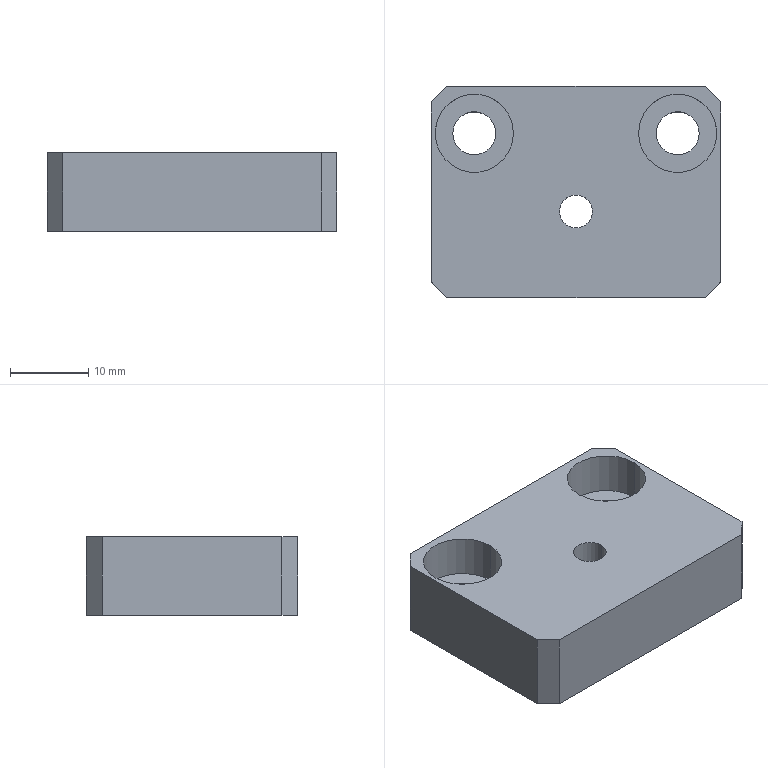Part | SolidWorks | features HoleWzd 2, Chamfer 1, Extrusion 1 | 1 solid | 22 faces | box 37 x 27 x 10 mm | volume 8705 mm3 | plane 12 | cylinder 10 | commonest cylinder face diameters 5.5 x4 10 x4 4.2 x2
STEP:
#1=CARTESIAN_POINT('',(-2.1,-2.5,0.));
#2=VERTEX_POINT('',#1);
#3=CARTESIAN_POINT('',(2.1,-2.5,0.));
#4=VERTEX_POINT('',#3);
#5=CARTESIAN_POINT('',(0.,-2.5,0.));
#6=DIRECTION('',(0.,0.,1.));
#7=DIRECTION('',(1.,0.,0.));
#8=AXIS2_PLACEMENT_3D('',#5,#6,#7);
#9=CIRCLE('',#8,2.1);
#10=EDGE_CURVE('',#2,#4,#9,.T.);
#11=ORIENTED_EDGE('',*,*,#10,.F.);
#12=CARTESIAN_POINT('',(-2.1,-2.5,10.));
#13=VERTEX_POINT('',#12);
#14=CARTESIAN_POINT('',(-2.1,-2.5,10.));
#15=DIRECTION('',(0.,0.,1.));
#16=VECTOR('',#15,1000.);
#17=LINE('',#14,#16);
#18=EDGE_CURVE('',#2,#13,#17,.T.);
#19=ORIENTED_EDGE('',*,*,#18,.T.);
#20=CARTESIAN_POINT('',(2.1,-2.5,10.));
#21=VERTEX_POINT('',#20);
#22=CARTESIAN_POINT('',(0.,-2.5,10.));
#23=DIRECTION('',(0.,0.,1.));
#24=DIRECTION('',(1.,0.,0.));
#25=AXIS2_PLACEMENT_3D('',#22,#23,#24);
#26=CIRCLE('',#25,2.1);
#27=EDGE_CURVE('',#13,#21,#26,.T.);
#28=ORIENTED_EDGE('',*,*,#27,.T.);
#29=CARTESIAN_POINT('',(2.1,-2.5,10.));
#30=DIRECTION('',(0.,0.,1.));
#31=VECTOR('',#30,1000.);
#32=LINE('',#29,#31);
#33=EDGE_CURVE('',#4,#21,#32,.T.);
#34=ORIENTED_EDGE('',*,*,#33,.F.);
#35=EDGE_LOOP('',(#11,#19,#28,#34));
#36=FACE_OUTER_BOUND('',#35,.T.);
#37=CARTESIAN_POINT('',(0.,-2.5,10.));
#38=DIRECTION('',(0.,0.,1.));
#39=DIRECTION('',(1.,0.,0.));
#40=AXIS2_PLACEMENT_3D('',#37,#38,#39);
#41=CYLINDRICAL_SURFACE('',#40,2.1);
#42=ADVANCED_FACE('',(#36),#41,.F.);
#43=CARTESIAN_POINT('',(-18.,7.5,4.6));
#44=VERTEX_POINT('',#43);
#45=CARTESIAN_POINT('',(-8.,7.5,4.6));
#46=VERTEX_POINT('',#45);
#47=CARTESIAN_POINT('',(-13.,7.5,4.6));
#48=DIRECTION('',(0.,0.,1.));
#49=DIRECTION('',(1.,0.,0.));
#50=AXIS2_PLACEMENT_3D('',#47,#48,#49);
#51=CIRCLE('',#50,5.);
#52=EDGE_CURVE('',#44,#46,#51,.T.);
#53=ORIENTED_EDGE('',*,*,#52,.F.);
#54=CARTESIAN_POINT('',(-18.,7.5,10.));
#55=VERTEX_POINT('',#54);
#56=CARTESIAN_POINT('',(-18.,7.5,10.));
#57=DIRECTION('',(0.,0.,1.));
#58=VECTOR('',#57,1000.);
#59=LINE('',#56,#58);
#60=EDGE_CURVE('',#44,#55,#59,.T.);
#61=ORIENTED_EDGE('',*,*,#60,.T.);
#62=CARTESIAN_POINT('',(-8.,7.5,10.));
#63=VERTEX_POINT('',#62);
#64=CARTESIAN_POINT('',(-13.,7.5,10.));
#65=DIRECTION('',(0.,0.,1.));
#66=DIRECTION('',(1.,0.,0.));
#67=AXIS2_PLACEMENT_3D('',#64,#65,#66);
#68=CIRCLE('',#67,5.);
#69=EDGE_CURVE('',#55,#63,#68,.T.);
#70=ORIENTED_EDGE('',*,*,#69,.T.);
#71=CARTESIAN_POINT('',(-8.,7.5,10.));
#72=DIRECTION('',(0.,0.,1.));
#73=VECTOR('',#72,1000.);
#74=LINE('',#71,#73);
#75=EDGE_CURVE('',#46,#63,#74,.T.);
#76=ORIENTED_EDGE('',*,*,#75,.F.);
#77=EDGE_LOOP('',(#53,#61,#70,#76));
#78=FACE_OUTER_BOUND('',#77,.T.);
#79=CARTESIAN_POINT('',(-13.,7.5,10.));
#80=DIRECTION('',(0.,0.,1.));
#81=DIRECTION('',(1.,0.,0.));
#82=AXIS2_PLACEMENT_3D('',#79,#80,#81);
#83=CYLINDRICAL_SURFACE('',#82,5.);
#84=ADVANCED_FACE('',(#78),#83,.F.);
#85=CARTESIAN_POINT('',(-15.75,7.5,0.));
#86=VERTEX_POINT('',#85);
#87=CARTESIAN_POINT('',(-10.25,7.5,0.));
#88=VERTEX_POINT('',#87);
#89=CARTESIAN_POINT('',(-13.,7.5,0.));
#90=DIRECTION('',(0.,0.,1.));
#91=DIRECTION('',(1.,0.,0.));
#92=AXIS2_PLACEMENT_3D('',#89,#90,#91);
#93=CIRCLE('',#92,2.75);
#94=EDGE_CURVE('',#86,#88,#93,.T.);
#95=ORIENTED_EDGE('',*,*,#94,.F.);
#96=CARTESIAN_POINT('',(-15.75,7.5,4.6));
#97=VERTEX_POINT('',#96);
#98=CARTESIAN_POINT('',(-15.75,7.5,10.));
#99=DIRECTION('',(0.,0.,1.));
#100=VECTOR('',#99,1000.);
#101=LINE('',#98,#100);
#102=EDGE_CURVE('',#86,#97,#101,.T.);
#103=ORIENTED_EDGE('',*,*,#102,.T.);
#104=CARTESIAN_POINT('',(-10.25,7.5,4.6));
#105=VERTEX_POINT('',#104);
#106=CARTESIAN_POINT('',(-13.,7.5,4.6));
#107=DIRECTION('',(0.,0.,1.));
#108=DIRECTION('',(1.,0.,0.));
#109=AXIS2_PLACEMENT_3D('',#106,#107,#108);
#110=CIRCLE('',#109,2.75);
#111=EDGE_CURVE('',#97,#105,#110,.T.);
#112=ORIENTED_EDGE('',*,*,#111,.T.);
#113=CARTESIAN_POINT('',(-10.25,7.5,10.));
#114=DIRECTION('',(0.,0.,1.));
#115=VECTOR('',#114,1000.);
#116=LINE('',#113,#115);
#117=EDGE_CURVE('',#88,#105,#116,.T.);
#118=ORIENTED_EDGE('',*,*,#117,.F.);
#119=EDGE_LOOP('',(#95,#103,#112,#118));
#120=FACE_OUTER_BOUND('',#119,.T.);
#121=CARTESIAN_POINT('',(-13.,7.5,10.));
#122=DIRECTION('',(0.,0.,1.));
#123=DIRECTION('',(1.,0.,0.));
#124=AXIS2_PLACEMENT_3D('',#121,#122,#123);
#125=CYLINDRICAL_SURFACE('',#124,2.75);
#126=ADVANCED_FACE('',(#120),#125,.F.);
#127=CARTESIAN_POINT('',(8.,7.5,4.6));
#128=VERTEX_POINT('',#127);
#129=CARTESIAN_POINT('',(18.,7.5,4.6));
#130=VERTEX_POINT('',#129);
#131=CARTESIAN_POINT('',(13.,7.5,4.6));
#132=DIRECTION('',(0.,0.,1.));
#133=DIRECTION('',(1.,0.,0.));
#134=AXIS2_PLACEMENT_3D('',#131,#132,#133);
#135=CIRCLE('',#134,5.);
#136=EDGE_CURVE('',#128,#130,#135,.T.);
#137=ORIENTED_EDGE('',*,*,#136,.F.);
#138=CARTESIAN_POINT('',(8.,7.5,10.));
#139=VERTEX_POINT('',#138);
#140=CARTESIAN_POINT('',(8.,7.5,10.));
#141=DIRECTION('',(0.,0.,1.));
#142=VECTOR('',#141,1000.);
#143=LINE('',#140,#142);
#144=EDGE_CURVE('',#128,#139,#143,.T.);
#145=ORIENTED_EDGE('',*,*,#144,.T.);
#146=CARTESIAN_POINT('',(18.,7.5,10.));
#147=VERTEX_POINT('',#146);
#148=CARTESIAN_POINT('',(13.,7.5,10.));
#149=DIRECTION('',(0.,0.,1.));
#150=DIRECTION('',(1.,0.,0.));
#151=AXIS2_PLACEMENT_3D('',#148,#149,#150);
#152=CIRCLE('',#151,5.);
#153=EDGE_CURVE('',#139,#147,#152,.T.);
#154=ORIENTED_EDGE('',*,*,#153,.T.);
#155=CARTESIAN_POINT('',(18.,7.5,10.));
#156=DIRECTION('',(0.,0.,1.));
#157=VECTOR('',#156,1000.);
#158=LINE('',#155,#157);
#159=EDGE_CURVE('',#130,#147,#158,.T.);
#160=ORIENTED_EDGE('',*,*,#159,.F.);
#161=EDGE_LOOP('',(#137,#145,#154,#160));
#162=FACE_OUTER_BOUND('',#161,.T.);
#163=CARTESIAN_POINT('',(13.,7.5,10.));
#164=DIRECTION('',(0.,0.,1.));
#165=DIRECTION('',(1.,0.,0.));
#166=AXIS2_PLACEMENT_3D('',#163,#164,#165);
#167=CYLINDRICAL_SURFACE('',#166,5.);
#168=ADVANCED_FACE('',(#162),#167,.F.);
#169=CARTESIAN_POINT('',(10.25,7.5,0.));
#170=VERTEX_POINT('',#169);
#171=CARTESIAN_POINT('',(15.75,7.5,0.));
#172=VERTEX_POINT('',#171);
#173=CARTESIAN_POINT('',(13.,7.5,0.));
#174=DIRECTION('',(0.,0.,1.));
#175=DIRECTION('',(1.,0.,0.));
#176=AXIS2_PLACEMENT_3D('',#173,#174,#175);
#177=CIRCLE('',#176,2.75);
#178=EDGE_CURVE('',#170,#172,#177,.T.);
#179=ORIENTED_EDGE('',*,*,#178,.F.);
#180=CARTESIAN_POINT('',(10.25,7.5,4.6));
#181=VERTEX_POINT('',#180);
#182=CARTESIAN_POINT('',(10.25,7.5,10.));
#183=DIRECTION('',(0.,0.,1.));
#184=VECTOR('',#183,1000.);
#185=LINE('',#182,#184);
#186=EDGE_CURVE('',#170,#181,#185,.T.);
#187=ORIENTED_EDGE('',*,*,#186,.T.);
#188=CARTESIAN_POINT('',(15.75,7.5,4.6));
#189=VERTEX_POINT('',#188);
#190=CARTESIAN_POINT('',(13.,7.5,4.6));
#191=DIRECTION('',(0.,0.,1.));
#192=DIRECTION('',(1.,0.,0.));
#193=AXIS2_PLACEMENT_3D('',#190,#191,#192);
#194=CIRCLE('',#193,2.75);
#195=EDGE_CURVE('',#181,#189,#194,.T.);
#196=ORIENTED_EDGE('',*,*,#195,.T.);
#197=CARTESIAN_POINT('',(15.75,7.5,10.));
#198=DIRECTION('',(0.,0.,1.));
#199=VECTOR('',#198,1000.);
#200=LINE('',#197,#199);
#201=EDGE_CURVE('',#172,#189,#200,.T.);
#202=ORIENTED_EDGE('',*,*,#201,.F.);
#203=EDGE_LOOP('',(#179,#187,#196,#202));
#204=FACE_OUTER_BOUND('',#203,.T.);
#205=CARTESIAN_POINT('',(13.,7.5,10.));
#206=DIRECTION('',(0.,0.,1.));
#207=DIRECTION('',(1.,0.,0.));
#208=AXIS2_PLACEMENT_3D('',#205,#206,#207);
#209=CYLINDRICAL_SURFACE('',#208,2.75);
#210=ADVANCED_FACE('',(#204),#209,.F.);
#211=CARTESIAN_POINT('',(18.5,-11.5,10.));
#212=VERTEX_POINT('',#211);
#213=CARTESIAN_POINT('',(18.5,11.5,10.));
#214=VERTEX_POINT('',#213);
#215=CARTESIAN_POINT('',(18.5,13.5,10.));
#216=DIRECTION('',(0.,1.,0.));
#217=VECTOR('',#216,1000.);
#218=LINE('',#215,#217);
#219=EDGE_CURVE('',#212,#214,#218,.T.);
#220=ORIENTED_EDGE('',*,*,#219,.F.);
#221=CARTESIAN_POINT('',(18.5,-11.5,0.));
#222=VERTEX_POINT('',#221);
#223=CARTESIAN_POINT('',(18.5,-11.5,10.));
#224=DIRECTION('',(0.,0.,-1.));
#225=VECTOR('',#224,1000.);
#226=LINE('',#223,#225);
#227=EDGE_CURVE('',#212,#222,#226,.T.);
#228=ORIENTED_EDGE('',*,*,#227,.T.);
#229=CARTESIAN_POINT('',(18.5,11.5,0.));
#230=VERTEX_POINT('',#229);
#231=CARTESIAN_POINT('',(18.5,13.5,0.));
#232=DIRECTION('',(0.,1.,0.));
#233=VECTOR('',#232,1000.);
#234=LINE('',#231,#233);
#235=EDGE_CURVE('',#222,#230,#234,.T.);
#236=ORIENTED_EDGE('',*,*,#235,.T.);
#237=CARTESIAN_POINT('',(18.5,11.5,10.));
#238=DIRECTION('',(0.,0.,1.));
#239=VECTOR('',#238,1000.);
#240=LINE('',#237,#239);
#241=EDGE_CURVE('',#230,#214,#240,.T.);
#242=ORIENTED_EDGE('',*,*,#241,.T.);
#243=EDGE_LOOP('',(#220,#228,#236,#242));
#244=FACE_OUTER_BOUND('',#243,.T.);
#245=CARTESIAN_POINT('',(18.5,13.5,10.));
#246=DIRECTION('',(-1.,0.,0.));
#247=DIRECTION('',(0.,-1.,0.));
#248=AXIS2_PLACEMENT_3D('',#245,#246,#247);
#249=PLANE('',#248);
#250=ADVANCED_FACE('',(#244),#249,.F.);
#251=CARTESIAN_POINT('',(16.5,13.5,10.));
#252=VERTEX_POINT('',#251);
#253=CARTESIAN_POINT('',(-16.5,13.5,10.));
#254=VERTEX_POINT('',#253);
#255=CARTESIAN_POINT('',(-18.5,13.5,10.));
#256=DIRECTION('',(-1.,0.,0.));
#257=VECTOR('',#256,1000.);
#258=LINE('',#255,#257);
#259=EDGE_CURVE('',#252,#254,#258,.T.);
#260=ORIENTED_EDGE('',*,*,#259,.F.);
#261=CARTESIAN_POINT('',(16.5,13.5,0.));
#262=VERTEX_POINT('',#261);
#263=CARTESIAN_POINT('',(16.5,13.5,10.));
#264=DIRECTION('',(0.,0.,-1.));
#265=VECTOR('',#264,1000.);
#266=LINE('',#263,#265);
#267=EDGE_CURVE('',#252,#262,#266,.T.);
#268=ORIENTED_EDGE('',*,*,#267,.T.);
#269=CARTESIAN_POINT('',(-16.5,13.5,0.));
#270=VERTEX_POINT('',#269);
#271=CARTESIAN_POINT('',(-18.5,13.5,0.));
#272=DIRECTION('',(-1.,0.,0.));
#273=VECTOR('',#272,1000.);
#274=LINE('',#271,#273);
#275=EDGE_CURVE('',#262,#270,#274,.T.);
#276=ORIENTED_EDGE('',*,*,#275,.T.);
#277=CARTESIAN_POINT('',(-16.5,13.5,10.));
#278=DIRECTION('',(0.,0.,1.));
#279=VECTOR('',#278,1000.);
#280=LINE('',#277,#279);
#281=EDGE_CURVE('',#270,#254,#280,.T.);
#282=ORIENTED_EDGE('',*,*,#281,.T.);
#283=EDGE_LOOP('',(#260,#268,#276,#282));
#284=FACE_OUTER_BOUND('',#283,.T.);
#285=CARTESIAN_POINT('',(-18.5,13.5,10.));
#286=DIRECTION('',(0.,-1.,0.));
#287=DIRECTION('',(0.,0.,-1.));
#288=AXIS2_PLACEMENT_3D('',#285,#286,#287);
#289=PLANE('',#288);
#290=ADVANCED_FACE('',(#284),#289,.F.);
#291=CARTESIAN_POINT('',(-18.5,11.5,0.));
#292=VERTEX_POINT('',#291);
#293=CARTESIAN_POINT('',(-18.5,-11.5,0.));
#294=VERTEX_POINT('',#293);
#295=CARTESIAN_POINT('',(-18.5,13.5,0.));
#296=DIRECTION('',(0.,-1.,0.));
#297=VECTOR('',#296,1000.);
#298=LINE('',#295,#297);
#299=EDGE_CURVE('',#292,#294,#298,.T.);
#300=ORIENTED_EDGE('',*,*,#299,.T.);
#301=CARTESIAN_POINT('',(-18.5,-11.5,10.));
#302=VERTEX_POINT('',#301);
#303=CARTESIAN_POINT('',(-18.5,-11.5,10.));
#304=DIRECTION('',(0.,0.,1.));
#305=VECTOR('',#304,1000.);
#306=LINE('',#303,#305);
#307=EDGE_CURVE('',#294,#302,#306,.T.);
#308=ORIENTED_EDGE('',*,*,#307,.T.);
#309=CARTESIAN_POINT('',(-18.5,11.5,10.));
#310=VERTEX_POINT('',#309);
#311=CARTESIAN_POINT('',(-18.5,13.5,10.));
#312=DIRECTION('',(0.,-1.,0.));
#313=VECTOR('',#312,1000.);
#314=LINE('',#311,#313);
#315=EDGE_CURVE('',#310,#302,#314,.T.);
#316=ORIENTED_EDGE('',*,*,#315,.F.);
#317=CARTESIAN_POINT('',(-18.5,11.5,10.));
#318=DIRECTION('',(0.,0.,-1.));
#319=VECTOR('',#318,1000.);
#320=LINE('',#317,#319);
#321=EDGE_CURVE('',#310,#292,#320,.T.);
#322=ORIENTED_EDGE('',*,*,#321,.T.);
#323=EDGE_LOOP('',(#300,#308,#316,#322));
#324=FACE_OUTER_BOUND('',#323,.T.);
#325=CARTESIAN_POINT('',(-18.5,13.5,10.));
#326=DIRECTION('',(1.,0.,0.));
#327=DIRECTION('',(0.,1.,0.));
#328=AXIS2_PLACEMENT_3D('',#325,#326,#327);
#329=PLANE('',#328);
#330=ADVANCED_FACE('',(#324),#329,.F.);
#331=CARTESIAN_POINT('',(-16.5,-13.5,10.));
#332=VERTEX_POINT('',#331);
#333=CARTESIAN_POINT('',(16.5,-13.5,10.));
#334=VERTEX_POINT('',#333);
#335=CARTESIAN_POINT('',(-18.5,-13.5,10.));
#336=DIRECTION('',(1.,0.,0.));
#337=VECTOR('',#336,1000.);
#338=LINE('',#335,#337);
#339=EDGE_CURVE('',#332,#334,#338,.T.);
#340=ORIENTED_EDGE('',*,*,#339,.F.);
#341=CARTESIAN_POINT('',(-16.5,-13.5,0.));
#342=VERTEX_POINT('',#341);
#343=CARTESIAN_POINT('',(-16.5,-13.5,10.));
#344=DIRECTION('',(0.,0.,-1.));
#345=VECTOR('',#344,1000.);
#346=LINE('',#343,#345);
#347=EDGE_CURVE('',#332,#342,#346,.T.);
#348=ORIENTED_EDGE('',*,*,#347,.T.);
#349=CARTESIAN_POINT('',(16.5,-13.5,0.));
#350=VERTEX_POINT('',#349);
#351=CARTESIAN_POINT('',(-18.5,-13.5,0.));
#352=DIRECTION('',(1.,0.,0.));
#353=VECTOR('',#352,1000.);
#354=LINE('',#351,#353);
#355=EDGE_CURVE('',#342,#350,#354,.T.);
#356=ORIENTED_EDGE('',*,*,#355,.T.);
#357=CARTESIAN_POINT('',(16.5,-13.5,10.));
#358=DIRECTION('',(0.,0.,1.));
#359=VECTOR('',#358,1000.);
#360=LINE('',#357,#359);
#361=EDGE_CURVE('',#350,#334,#360,.T.);
#362=ORIENTED_EDGE('',*,*,#361,.T.);
#363=EDGE_LOOP('',(#340,#348,#356,#362));
#364=FACE_OUTER_BOUND('',#363,.T.);
#365=CARTESIAN_POINT('',(-18.5,-13.5,10.));
#366=DIRECTION('',(0.,1.,0.));
#367=DIRECTION('',(0.,0.,1.));
#368=AXIS2_PLACEMENT_3D('',#365,#366,#367);
#369=PLANE('',#368);
#370=ADVANCED_FACE('',(#364),#369,.F.);
#371=CARTESIAN_POINT('',(0.,-2.5,10.));
#372=DIRECTION('',(0.,0.,1.));
#373=DIRECTION('',(1.,0.,0.));
#374=AXIS2_PLACEMENT_3D('',#371,#372,#373);
#375=CIRCLE('',#374,2.1);
#376=EDGE_CURVE('',#21,#13,#375,.T.);
#377=ORIENTED_EDGE('',*,*,#376,.F.);
#378=ORIENTED_EDGE('',*,*,#27,.F.);
#379=EDGE_LOOP('',(#377,#378));
#380=FACE_BOUND('',#379,.T.);
#381=CARTESIAN_POINT('',(-13.,7.5,10.));
#382=DIRECTION('',(0.,0.,1.));
#383=DIRECTION('',(1.,0.,0.));
#384=AXIS2_PLACEMENT_3D('',#381,#382,#383);
#385=CIRCLE('',#384,5.);
#386=EDGE_CURVE('',#63,#55,#385,.T.);
#387=ORIENTED_EDGE('',*,*,#386,.F.);
#388=ORIENTED_EDGE('',*,*,#69,.F.);
#389=EDGE_LOOP('',(#387,#388));
#390=FACE_BOUND('',#389,.T.);
#391=CARTESIAN_POINT('',(13.,7.5,10.));
#392=DIRECTION('',(0.,0.,1.));
#393=DIRECTION('',(1.,0.,0.));
#394=AXIS2_PLACEMENT_3D('',#391,#392,#393);
#395=CIRCLE('',#394,5.);
#396=EDGE_CURVE('',#147,#139,#395,.T.);
#397=ORIENTED_EDGE('',*,*,#396,.F.);
#398=ORIENTED_EDGE('',*,*,#153,.F.);
#399=EDGE_LOOP('',(#397,#398));
#400=FACE_BOUND('',#399,.T.);
#401=ORIENTED_EDGE('',*,*,#315,.T.);
#402=CARTESIAN_POINT('',(-15.,-15.,10.));
#403=DIRECTION('',(0.7071,-0.7071,0.));
#404=VECTOR('',#403,1000.);
#405=LINE('',#402,#404);
#406=EDGE_CURVE('',#302,#332,#405,.T.);
#407=ORIENTED_EDGE('',*,*,#406,.T.);
#408=ORIENTED_EDGE('',*,*,#339,.T.);
#409=CARTESIAN_POINT('',(15.,-15.,10.));
#410=DIRECTION('',(0.7071,0.7071,0.));
#411=VECTOR('',#410,1000.);
#412=LINE('',#409,#411);
#413=EDGE_CURVE('',#334,#212,#412,.T.);
#414=ORIENTED_EDGE('',*,*,#413,.T.);
#415=ORIENTED_EDGE('',*,*,#219,.T.);
#416=CARTESIAN_POINT('',(15.,15.,10.));
#417=DIRECTION('',(-0.7071,0.7071,0.));
#418=VECTOR('',#417,1000.);
#419=LINE('',#416,#418);
#420=EDGE_CURVE('',#214,#252,#419,.T.);
#421=ORIENTED_EDGE('',*,*,#420,.T.);
#422=ORIENTED_EDGE('',*,*,#259,.T.);
#423=CARTESIAN_POINT('',(-15.,15.,10.));
#424=DIRECTION('',(-0.7071,-0.7071,0.));
#425=VECTOR('',#424,1000.);
#426=LINE('',#423,#425);
#427=EDGE_CURVE('',#254,#310,#426,.T.);
#428=ORIENTED_EDGE('',*,*,#427,.T.);
#429=EDGE_LOOP('',(#401,#407,#408,#414,#415,#421,#422,#428));
#430=FACE_OUTER_BOUND('',#429,.T.);
#431=CARTESIAN_POINT('',(0.,0.,10.));
#432=DIRECTION('',(0.,0.,1.));
#433=DIRECTION('',(1.,0.,0.));
#434=AXIS2_PLACEMENT_3D('',#431,#432,#433);
#435=PLANE('',#434);
#436=ADVANCED_FACE('',(#380,#390,#400,#430),#435,.T.);
#437=CARTESIAN_POINT('',(0.,-2.5,0.));
#438=DIRECTION('',(0.,0.,1.));
#439=DIRECTION('',(1.,0.,0.));
#440=AXIS2_PLACEMENT_3D('',#437,#438,#439);
#441=CIRCLE('',#440,2.1);
#442=EDGE_CURVE('',#4,#2,#441,.T.);
#443=ORIENTED_EDGE('',*,*,#442,.T.);
#444=ORIENTED_EDGE('',*,*,#10,.T.);
#445=EDGE_LOOP('',(#443,#444));
#446=FACE_BOUND('',#445,.T.);
#447=CARTESIAN_POINT('',(-13.,7.5,0.));
#448=DIRECTION('',(0.,0.,1.));
#449=DIRECTION('',(1.,0.,0.));
#450=AXIS2_PLACEMENT_3D('',#447,#448,#449);
#451=CIRCLE('',#450,2.75);
#452=EDGE_CURVE('',#88,#86,#451,.T.);
#453=ORIENTED_EDGE('',*,*,#452,.T.);
#454=ORIENTED_EDGE('',*,*,#94,.T.);
#455=EDGE_LOOP('',(#453,#454));
#456=FACE_BOUND('',#455,.T.);
#457=CARTESIAN_POINT('',(13.,7.5,0.));
#458=DIRECTION('',(0.,0.,1.));
#459=DIRECTION('',(1.,0.,0.));
#460=AXIS2_PLACEMENT_3D('',#457,#458,#459);
#461=CIRCLE('',#460,2.75);
#462=EDGE_CURVE('',#172,#170,#461,.T.);
#463=ORIENTED_EDGE('',*,*,#462,.T.);
#464=ORIENTED_EDGE('',*,*,#178,.T.);
#465=EDGE_LOOP('',(#463,#464));
#466=FACE_BOUND('',#465,.T.);
#467=ORIENTED_EDGE('',*,*,#355,.F.);
#468=CARTESIAN_POINT('',(-16.5,-13.5,0.));
#469=DIRECTION('',(-0.7071,0.7071,0.));
#470=VECTOR('',#469,1000.);
#471=LINE('',#468,#470);
#472=EDGE_CURVE('',#342,#294,#471,.T.);
#473=ORIENTED_EDGE('',*,*,#472,.T.);
#474=ORIENTED_EDGE('',*,*,#299,.F.);
#475=CARTESIAN_POINT('',(-18.5,11.5,0.));
#476=DIRECTION('',(0.7071,0.7071,0.));
#477=VECTOR('',#476,1000.);
#478=LINE('',#475,#477);
#479=EDGE_CURVE('',#292,#270,#478,.T.);
#480=ORIENTED_EDGE('',*,*,#479,.T.);
#481=ORIENTED_EDGE('',*,*,#275,.F.);
#482=CARTESIAN_POINT('',(16.5,13.5,0.));
#483=DIRECTION('',(0.7071,-0.7071,0.));
#484=VECTOR('',#483,1000.);
#485=LINE('',#482,#484);
#486=EDGE_CURVE('',#262,#230,#485,.T.);
#487=ORIENTED_EDGE('',*,*,#486,.T.);
#488=ORIENTED_EDGE('',*,*,#235,.F.);
#489=CARTESIAN_POINT('',(18.5,-11.5,0.));
#490=DIRECTION('',(-0.7071,-0.7071,0.));
#491=VECTOR('',#490,1000.);
#492=LINE('',#489,#491);
#493=EDGE_CURVE('',#222,#350,#492,.T.);
#494=ORIENTED_EDGE('',*,*,#493,.T.);
#495=EDGE_LOOP('',(#467,#473,#474,#480,#481,#487,#488,#494));
#496=FACE_OUTER_BOUND('',#495,.T.);
#497=CARTESIAN_POINT('',(0.,0.,0.));
#498=DIRECTION('',(0.,0.,1.));
#499=DIRECTION('',(1.,0.,0.));
#500=AXIS2_PLACEMENT_3D('',#497,#498,#499);
#501=PLANE('',#500);
#502=ADVANCED_FACE('',(#446,#456,#466,#496),#501,.F.);
#503=ORIENTED_EDGE('',*,*,#186,.F.);
#504=ORIENTED_EDGE('',*,*,#462,.F.);
#505=ORIENTED_EDGE('',*,*,#201,.T.);
#506=CARTESIAN_POINT('',(13.,7.5,4.6));
#507=DIRECTION('',(0.,0.,1.));
#508=DIRECTION('',(1.,0.,0.));
#509=AXIS2_PLACEMENT_3D('',#506,#507,#508);
#510=CIRCLE('',#509,2.75);
#511=EDGE_CURVE('',#189,#181,#510,.T.);
#512=ORIENTED_EDGE('',*,*,#511,.T.);
#513=EDGE_LOOP('',(#503,#504,#505,#512));
#514=FACE_OUTER_BOUND('',#513,.T.);
#515=CARTESIAN_POINT('',(13.,7.5,10.));
#516=DIRECTION('',(0.,0.,1.));
#517=DIRECTION('',(1.,0.,0.));
#518=AXIS2_PLACEMENT_3D('',#515,#516,#517);
#519=CYLINDRICAL_SURFACE('',#518,2.75);
#520=ADVANCED_FACE('',(#514),#519,.F.);
#521=ORIENTED_EDGE('',*,*,#511,.F.);
#522=ORIENTED_EDGE('',*,*,#195,.F.);
#523=EDGE_LOOP('',(#521,#522));
#524=FACE_BOUND('',#523,.T.);
#525=CARTESIAN_POINT('',(13.,7.5,4.6));
#526=DIRECTION('',(0.,0.,1.));
#527=DIRECTION('',(1.,0.,0.));
#528=AXIS2_PLACEMENT_3D('',#525,#526,#527);
#529=CIRCLE('',#528,5.);
#530=EDGE_CURVE('',#130,#128,#529,.T.);
#531=ORIENTED_EDGE('',*,*,#530,.T.);
#532=ORIENTED_EDGE('',*,*,#136,.T.);
#533=EDGE_LOOP('',(#531,#532));
#534=FACE_OUTER_BOUND('',#533,.T.);
#535=CARTESIAN_POINT('',(15.75,7.5,4.6));
#536=DIRECTION('',(0.,0.,-1.));
#537=DIRECTION('',(-1.,0.,0.));
#538=AXIS2_PLACEMENT_3D('',#535,#536,#537);
#539=PLANE('',#538);
#540=ADVANCED_FACE('',(#524,#534),#539,.F.);
#541=ORIENTED_EDGE('',*,*,#144,.F.);
#542=ORIENTED_EDGE('',*,*,#530,.F.);
#543=ORIENTED_EDGE('',*,*,#159,.T.);
#544=ORIENTED_EDGE('',*,*,#396,.T.);
#545=EDGE_LOOP('',(#541,#542,#543,#544));
#546=FACE_OUTER_BOUND('',#545,.T.);
#547=CARTESIAN_POINT('',(13.,7.5,10.));
#548=DIRECTION('',(0.,0.,1.));
#549=DIRECTION('',(1.,0.,0.));
#550=AXIS2_PLACEMENT_3D('',#547,#548,#549);
#551=CYLINDRICAL_SURFACE('',#550,5.);
#552=ADVANCED_FACE('',(#546),#551,.F.);
#553=ORIENTED_EDGE('',*,*,#102,.F.);
#554=ORIENTED_EDGE('',*,*,#452,.F.);
#555=ORIENTED_EDGE('',*,*,#117,.T.);
#556=CARTESIAN_POINT('',(-13.,7.5,4.6));
#557=DIRECTION('',(0.,0.,1.));
#558=DIRECTION('',(1.,0.,0.));
#559=AXIS2_PLACEMENT_3D('',#556,#557,#558);
#560=CIRCLE('',#559,2.75);
#561=EDGE_CURVE('',#105,#97,#560,.T.);
#562=ORIENTED_EDGE('',*,*,#561,.T.);
#563=EDGE_LOOP('',(#553,#554,#555,#562));
#564=FACE_OUTER_BOUND('',#563,.T.);
#565=CARTESIAN_POINT('',(-13.,7.5,10.));
#566=DIRECTION('',(0.,0.,1.));
#567=DIRECTION('',(1.,0.,0.));
#568=AXIS2_PLACEMENT_3D('',#565,#566,#567);
#569=CYLINDRICAL_SURFACE('',#568,2.75);
#570=ADVANCED_FACE('',(#564),#569,.F.);
#571=ORIENTED_EDGE('',*,*,#561,.F.);
#572=ORIENTED_EDGE('',*,*,#111,.F.);
#573=EDGE_LOOP('',(#571,#572));
#574=FACE_BOUND('',#573,.T.);
#575=CARTESIAN_POINT('',(-13.,7.5,4.6));
#576=DIRECTION('',(0.,0.,1.));
#577=DIRECTION('',(1.,0.,0.));
#578=AXIS2_PLACEMENT_3D('',#575,#576,#577);
#579=CIRCLE('',#578,5.);
#580=EDGE_CURVE('',#46,#44,#579,.T.);
#581=ORIENTED_EDGE('',*,*,#580,.T.);
#582=ORIENTED_EDGE('',*,*,#52,.T.);
#583=EDGE_LOOP('',(#581,#582));
#584=FACE_OUTER_BOUND('',#583,.T.);
#585=CARTESIAN_POINT('',(-10.25,7.5,4.6));
#586=DIRECTION('',(0.,0.,-1.));
#587=DIRECTION('',(-1.,0.,0.));
#588=AXIS2_PLACEMENT_3D('',#585,#586,#587);
#589=PLANE('',#588);
#590=ADVANCED_FACE('',(#574,#584),#589,.F.);
#591=ORIENTED_EDGE('',*,*,#60,.F.);
#592=ORIENTED_EDGE('',*,*,#580,.F.);
#593=ORIENTED_EDGE('',*,*,#75,.T.);
#594=ORIENTED_EDGE('',*,*,#386,.T.);
#595=EDGE_LOOP('',(#591,#592,#593,#594));
#596=FACE_OUTER_BOUND('',#595,.T.);
#597=CARTESIAN_POINT('',(-13.,7.5,10.));
#598=DIRECTION('',(0.,0.,1.));
#599=DIRECTION('',(1.,0.,0.));
#600=AXIS2_PLACEMENT_3D('',#597,#598,#599);
#601=CYLINDRICAL_SURFACE('',#600,5.);
#602=ADVANCED_FACE('',(#596),#601,.F.);
#603=ORIENTED_EDGE('',*,*,#18,.F.);
#604=ORIENTED_EDGE('',*,*,#442,.F.);
#605=ORIENTED_EDGE('',*,*,#33,.T.);
#606=ORIENTED_EDGE('',*,*,#376,.T.);
#607=EDGE_LOOP('',(#603,#604,#605,#606));
#608=FACE_OUTER_BOUND('',#607,.T.);
#609=CARTESIAN_POINT('',(0.,-2.5,10.));
#610=DIRECTION('',(0.,0.,1.));
#611=DIRECTION('',(1.,0.,0.));
#612=AXIS2_PLACEMENT_3D('',#609,#610,#611);
#613=CYLINDRICAL_SURFACE('',#612,2.1);
#614=ADVANCED_FACE('',(#608),#613,.F.);
#615=ORIENTED_EDGE('',*,*,#406,.F.);
#616=ORIENTED_EDGE('',*,*,#307,.F.);
#617=ORIENTED_EDGE('',*,*,#472,.F.);
#618=ORIENTED_EDGE('',*,*,#347,.F.);
#619=EDGE_LOOP('',(#615,#616,#617,#618));
#620=FACE_OUTER_BOUND('',#619,.T.);
#621=CARTESIAN_POINT('',(-16.5,-13.5,10.));
#622=DIRECTION('',(0.7071,0.7071,0.));
#623=DIRECTION('',(0.,0.,-1.));
#624=AXIS2_PLACEMENT_3D('',#621,#622,#623);
#625=PLANE('',#624);
#626=ADVANCED_FACE('',(#620),#625,.F.);
#627=ORIENTED_EDGE('',*,*,#413,.F.);
#628=ORIENTED_EDGE('',*,*,#361,.F.);
#629=ORIENTED_EDGE('',*,*,#493,.F.);
#630=ORIENTED_EDGE('',*,*,#227,.F.);
#631=EDGE_LOOP('',(#627,#628,#629,#630));
#632=FACE_OUTER_BOUND('',#631,.T.);
#633=CARTESIAN_POINT('',(18.5,-11.5,10.));
#634=DIRECTION('',(-0.7071,0.7071,0.));
#635=DIRECTION('',(0.,0.,-1.));
#636=AXIS2_PLACEMENT_3D('',#633,#634,#635);
#637=PLANE('',#636);
#638=ADVANCED_FACE('',(#632),#637,.F.);
#639=ORIENTED_EDGE('',*,*,#420,.F.);
#640=ORIENTED_EDGE('',*,*,#241,.F.);
#641=ORIENTED_EDGE('',*,*,#486,.F.);
#642=ORIENTED_EDGE('',*,*,#267,.F.);
#643=EDGE_LOOP('',(#639,#640,#641,#642));
#644=FACE_OUTER_BOUND('',#643,.T.);
#645=CARTESIAN_POINT('',(16.5,13.5,10.));
#646=DIRECTION('',(-0.7071,-0.7071,0.));
#647=DIRECTION('',(0.,0.,-1.));
#648=AXIS2_PLACEMENT_3D('',#645,#646,#647);
#649=PLANE('',#648);
#650=ADVANCED_FACE('',(#644),#649,.F.);
#651=ORIENTED_EDGE('',*,*,#427,.F.);
#652=ORIENTED_EDGE('',*,*,#281,.F.);
#653=ORIENTED_EDGE('',*,*,#479,.F.);
#654=ORIENTED_EDGE('',*,*,#321,.F.);
#655=EDGE_LOOP('',(#651,#652,#653,#654));
#656=FACE_OUTER_BOUND('',#655,.T.);
#657=CARTESIAN_POINT('',(-18.5,11.5,10.));
#658=DIRECTION('',(0.7071,-0.7071,0.));
#659=DIRECTION('',(0.,0.,-1.));
#660=AXIS2_PLACEMENT_3D('',#657,#658,#659);
#661=PLANE('',#660);
#662=ADVANCED_FACE('',(#656),#661,.F.);
#663=CLOSED_SHELL('',(#42,#84,#126,#168,#210,#250,#290,#330,#370,#436,#502,#520,#540,#552,#570,#590,#602,#614,#626,#638,#650,#662));
#664=MANIFOLD_SOLID_BREP('',#663);
#665=CARTESIAN_POINT('',(0.,0.,0.));
#666=DIRECTION('',(0.,0.,1.));
#667=DIRECTION('',(1.,0.,0.));
#668=AXIS2_PLACEMENT_3D('',#665,#666,#667);
#669=(LENGTH_UNIT()NAMED_UNIT(*)SI_UNIT(.MILLI.,.METRE.));
#670=UNCERTAINTY_MEASURE_WITH_UNIT(LENGTH_MEASURE(0.00001),#669,'','');
#671=(NAMED_UNIT(*)PLANE_ANGLE_UNIT()SI_UNIT($,.RADIAN.));
#672=(NAMED_UNIT(*)SI_UNIT($,.STERADIAN.)SOLID_ANGLE_UNIT());
#673=(GEOMETRIC_REPRESENTATION_CONTEXT(3)GLOBAL_UNCERTAINTY_ASSIGNED_CONTEXT((#670))GLOBAL_UNIT_ASSIGNED_CONTEXT((#669,#671,#672))REPRESENTATION_CONTEXT('',''));
#674=ADVANCED_BREP_SHAPE_REPRESENTATION('',(#664,#668),#673);